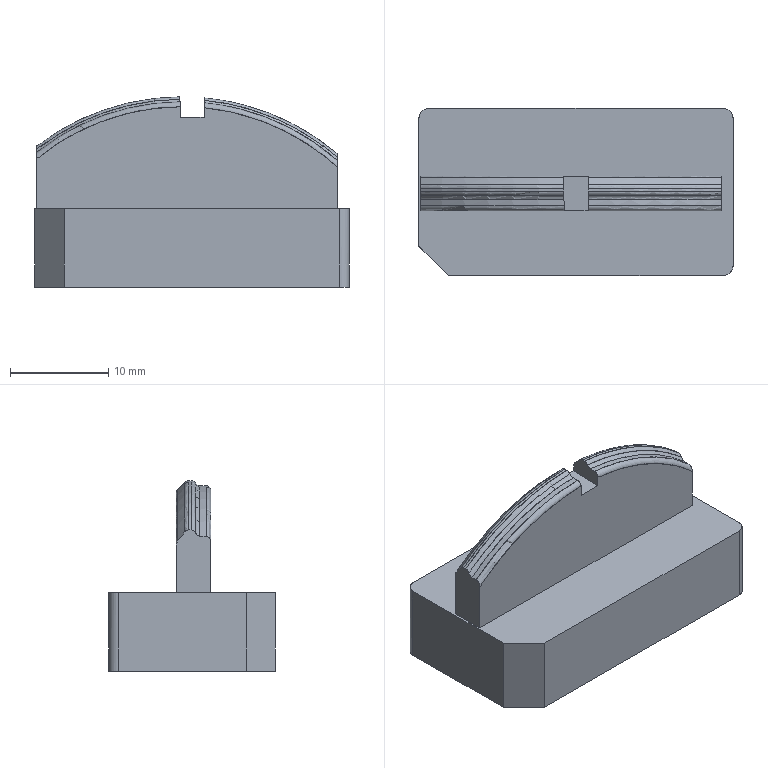NC program | PowerMill | posted with a generic post | part box 32 x 17 x 19.383 mm
Lines 3866 to 4878 of 94163:
N3963 M6
N3964 S18000 M03
N3965 G00 G90 X0.0 Y0.0
N3966 G43 Z9.8028 H2
N3967
N3968 G05 P10000 R4
N3969 X-3.7476 Y3.5833
N3970 Z0.7947
N3971 G01 Z-0.4053 F3600.0
N3972 X-3.7563 Y3.5631 F6000.0
N3973 G03 X-3.6536 Y3.3027 I0.1816 J-0.0788
N3974 G01 X-2.338 Y2.7316
N3975 X-1.4642 Y2.779
N3976 X-0.9761 Y2.7673
N3977 X-0.4881 Y2.6348
N3978 X0.0 Y2.3461
N3979 G03 X0.2177 Y2.3492 I0.1064 J0.1712
N3980 G01 X0.4881 Y2.5054
N3981 X0.9761 Y2.6463
N3982 X1.4642 Y2.6614
N3983 X1.9522 Y2.5817
N3984 X2.4403 Y2.4561
N3985 X2.9283 Y2.272
N3986 X3.0642 Y2.1962
N3987 X3.4164 Y1.9204
N3988 X3.6343 Y1.7082
N3989 X3.9586 Y1.2201
N3990 X4.1158 Y0.7321
N3991 X4.1454 Y0.244
N3992 X4.1238 Y-0.244
N3993 X3.9806 Y-0.7321
N3994 X3.6681 Y-1.2201
N3995 X3.4164 Y-1.4774
N3996 X3.1409 Y-1.7082
N3997 X2.9283 Y-1.8324
N3998 X2.4403 Y-2.0184
N3999 X1.9522 Y-2.1453
N4000 X1.6527 Y-2.1962
N4001 X1.4642 Y-2.2234
N4002 X0.9761 Y-2.2126
N4003 X0.4881 Y-2.076
N4004 X0.1844 Y-1.9036
N4005 X0.0824 Y-1.8775
N4006 X-0.0187 Y-1.9069
N4007 X-0.4881 Y-2.1938
N4008 X-0.9761 Y-2.3211
N4009 X-1.4642 Y-2.3318
N4010 X-2.4403 Y-2.3036
N4011 X-3.9044 Y-2.1592
N4012 X-4.3925 Y-2.0308
N4013 X-4.8805 Y-1.8556
N4014 X-5.134 Y-1.7082
N4015 X-5.6952 Y-1.2201
N4016 X-5.9992 Y-0.7321
N4017 X-6.1407 Y-0.244
N4018 X-6.1636 Y0.244
N4019 X-6.1312 Y0.7321
N4020 X-5.976 Y1.2201
N4021 X-5.6491 Y1.7082
N4022 X-5.3686 Y1.9608
N4023 X-5.0595 Y2.1962
N4024 X-4.8805 Y2.2928
N4025 X-4.3925 Y2.4695
N4026 X-3.9044 Y2.5972
N4027 X-3.2118 Y2.6843
N4028 X-2.338 Y2.7316
N4029 X-3.7478 Y3.8043 Z-0.6036
N4030 X-3.7567 Y3.7842
N4031 G03 X-3.6566 Y3.5227 I0.1808 J-0.0806
N4032 G01 X-2.3471 Y2.9385
N4033 X-1.4642 Y2.9774
N4034 X-0.9761 Y2.965
N4035 X-0.4881 Y2.8316
N4036 X-0.2016 Y2.6843
N4037 X-0.026 Y2.5528
N4038 G03 X0.1946 Y2.5402 I0.1198 J0.1601
N4039 G01 X0.4881 Y2.7114
N4040 X0.9761 Y2.8532
N4041 X1.4642 Y2.8693
N4042 X2.9283 Y2.6859
N4043 X3.4164 Y2.5799
N4044 X3.9044 Y2.4176
N4045 X4.3925 Y2.1844
N4046 X4.8805 Y1.7486
N4047 X5.241 Y1.2201
N4048 X5.3967 Y0.7321
N4049 X5.4278 Y0.244
N4050 X5.4058 Y-0.244
N4051 X5.2581 Y-0.7321
N4052 X4.9589 Y-1.2201
N4053 X4.4471 Y-1.7082
N4054 X3.9044 Y-1.9782
N4055 X3.4164 Y-2.1392
N4056 X3.16 Y-2.1962
N4057 X2.9283 Y-2.2438
N4058 X1.4642 Y-2.3989
N4059 X0.9761 Y-2.3887
N4060 X0.4881 Y-2.2532
N4061 X0.201 Y-2.0907
N4062 X0.0946 Y-2.065
N4063 X-0.0096 Y-2.0985
N4064 X-0.4881 Y-2.3712
N4065 X-0.9761 Y-2.4979
N4066 X-1.4642 Y-2.5012
N4067 X-2.9283 Y-2.4374
N4068 X-4.8805 Y-2.2565
N4069 X-5.1745 Y-2.1962
N4070 X-5.8566 Y-1.9976
N4071 X-6.442 Y-1.7082
N4072 X-6.8327 Y-1.3532
N4073 X-7.2418 Y-0.7321
N4074 X-7.3839 Y-0.244
N4075 X-7.4067 Y0.244
N4076 X-7.3776 Y0.7321
N4077 X-7.2204 Y1.2201
N4078 X-6.9008 Y1.7082
N4079 X-6.3684 Y2.1962
N4080 X-5.8566 Y2.4347
N4081 X-5.3686 Y2.5917
N4082 X-4.9434 Y2.6843
N4083 X-2.9283 Y2.9129
N4084 X-2.3471 Y2.9385
N4085 G00 Z3.3981
N4086 G01 X0.9211 Y-3.7408 F10000.0
N4087 G00 Z0.3981
N4088 G01 Z-0.8019 F3600.0
N4089 X0.9265 Y-3.7195 F6000.0
N4090 G03 X0.7832 Y-3.4789 I-0.1919 J0.0487
N4091 G01 X0.4881 Y-3.404
N4092 X0.2671 Y-3.2865
N4093 G03 X0.0461 Y-3.3086 I-0.0939 J-0.1765
N4094 G01 X0.0 Y-3.3465
N4095 X-0.4881 Y-3.6181
N4096 X-0.6096 Y-3.6604
N4097 X-0.9761 Y-3.7392
N4098 X-1.4642 Y-3.7429
N4099 X-2.4403 Y-3.6987
N4100 X-3.4164 Y-3.5562
N4101 X-3.9044 Y-3.4048
N4102 X-4.2369 Y-3.2391
N4103 X-4.4587 Y-3.7227
N4104 X-4.3614 Y-3.6007
N4105 G03 X-4.4127 Y-3.1454 I-0.2533 J0.2021
N4106 G01 X-4.8805 Y-2.7721
N4107 X-4.9173 Y-2.7232
N4108 X-4.9604 Y-2.6796
N4109 X-5.1023 Y-2.4674
N4110 X-5.1612 Y-2.4098
N4111 X-5.2383 Y-2.3809
N4112 X-6.3447 Y-2.2115
N4113 X-6.8327 Y-2.0687
N4114 X-7.3208 Y-1.836
N4115 X-7.5374 Y-1.7082
N4116 X-7.8088 Y-1.4798
N4117 X-8.0321 Y-1.2201
N4118 X-8.2969 Y-0.7807
N4119 X-8.4632 Y-0.244
N4120 X-8.4838 Y0.244
N4121 X-8.4563 Y0.7321
N4122 X-8.2975 Y1.2201
N4123 X-7.9964 Y1.7082
N4124 X-7.8088 Y1.9185
N4125 X-7.4608 Y2.1962
N4126 X-6.8327 Y2.5063
N4127 X-6.3447 Y2.6533
N4128 X-4.8805 Y2.9144
N4129 X-2.9283 Y3.1355
N4130 X-1.4642 Y3.2002
N4131 X-0.9761 Y3.1871
N4132 X-0.4881 Y3.0526
N4133 X-0.0037 Y2.7633
N4134 X0.0979 Y2.735
N4135 X0.1999 Y2.7624
N4136 X0.4881 Y2.931
N4137 X0.9761 Y3.0739
N4138 X1.4642 Y3.0909
N4139 X2.9283 Y2.9063
N4140 X4.1964 Y2.6843
N4141 X4.8805 Y2.4874
N4142 X5.3686 Y2.2533
N4143 X5.8566 Y1.8745
N4144 X6.0012 Y1.7082
N4145 X6.3138 Y1.2201
N4146 X6.4711 Y0.7321
N4147 X6.5027 Y0.244
N4148 X6.4766 Y-0.244
N4149 X6.3447 Y-0.7097
N4150 X6.0361 Y-1.2201
N4151 X5.8566 Y-1.4383
N4152 X5.5407 Y-1.7082
N4153 X4.8805 Y-2.0491
N4154 X4.3925 Y-2.1953
N4155 X3.9044 Y-2.2952
N4156 X3.2179 Y-2.3924
N4157 X3.1399 Y-2.4209
N4158 X3.0801 Y-2.4786
N4159 X2.9454 Y-2.6783
N4160 X2.673 Y-2.9433
N4161 X4.0519 Y-4.1006 Z-1.0002
N4162 X4.0568 Y-4.0792
N4163 G03 X3.9087 Y-3.8416 I-0.1928 J0.0448
N4164 G01 X2.8287 Y-3.5911
N4165 X2.5403 Y-3.6604
N4166 X1.4642 Y-3.8057
N4167 X0.9761 Y-3.8028
N4168 X0.4582 Y-3.6604
N4169 X0.1659 Y-3.4944
N4170 X0.0607 Y-3.4684
N4171 X-0.0425 Y-3.501
N4172 X-0.2857 Y-3.6604
N4173 X-0.4881 Y-3.7513
N4174 X-0.9761 Y-3.8705
N4175 X-2.4403 Y-3.8583
N4176 X-3.4164 Y-3.8055
N4177 X-4.5237 Y-3.6604
N4178 X-5.3686 Y-3.4189
N4179 X-5.7942 Y-3.1723
N4180 X-6.2938 Y-2.6843
N4181 X-6.4777 Y-2.3999
N4182 X-6.5331 Y-2.3432
N4183 X-6.6062 Y-2.3124
N4184 X-7.1834 Y-2.1962
N4185 X-7.8088 Y-1.9767
N4186 X-8.2543 Y-1.7082
N4187 X-8.7521 Y-1.2201
N4188 X-9.0335 Y-0.7321
N4189 X-9.1759 Y-0.244
N4190 X-9.1994 Y0.244
N4191 X-9.1698 Y0.7321
N4192 X-9.0126 Y1.2201
N4193 X-8.7148 Y1.7082
N4194 X-8.2969 Y2.1169
N4195 X-7.8088 Y2.4151
N4196 X-7.3208 Y2.596
N4197 X-6.3447 Y2.8264
N4198 X-4.8805 Y3.0857
N4199 X-2.9283 Y3.3093
N4200 X-1.4642 Y3.3742
N4201 X-0.9761 Y3.3605
N4202 X-0.4881 Y3.2252
N4203 X-0.3728 Y3.1723
N4204 X-0.0239 Y2.9344
N4205 G03 X0.1902 Y2.9273 I0.1127 J0.1653
N4206 G01 X0.4881 Y3.1025
N4207 X0.9761 Y3.2462
N4208 X1.4642 Y3.264
N4209 X2.9283 Y3.0789
N4210 X5.0066 Y2.6843
N4211 X5.3686 Y2.5799
N4212 X5.8566 Y2.3869
N4213 X6.3447 Y2.0755
N4214 X6.709 Y1.7082
N4215 X6.9935 Y1.2201
N4216 X7.1505 Y0.7321
N4217 X7.1803 Y0.244
N4218 X7.1592 Y-0.244
N4219 X7.0157 Y-0.7321
N4220 X6.7468 Y-1.2201
N4221 X6.3447 Y-1.639
N4222 X5.8566 Y-1.9491
N4223 X5.192 Y-2.1962
N4224 X4.6142 Y-2.3093
N4225 X4.5353 Y-2.3437
N4226 X4.4777 Y-2.4077
N4227 X4.298 Y-2.6843
N4228 X3.7785 Y-3.1723
N4229 X3.4164 Y-3.3918
N4230 X2.9283 Y-3.5672
N4231 X2.8287 Y-3.5911
N4232 X4.0743 Y-4.5766 Z-1.1985
N4233 X4.0829 Y-4.5564
N4234 G03 X3.9773 Y-4.297 I-0.1825 J0.0769
N4235 G01 X2.8435 Y-3.8193
N4236 X1.4642 Y-3.9089
N4237 X0.9761 Y-3.8976
N4238 X0.4881 Y-3.7699
N4239 X0.2603 Y-3.6604
N4240 X0.1365 Y-3.5794
N4241 G03 X-0.0964 Y-3.5886 I-0.1099 J-0.1689
N4242 G01 X-0.2035 Y-3.6604
N4243 X-0.4881 Y-3.7962
N4244 X-0.9761 Y-3.9159
N4245 X-3.4164 Y-3.908
N4246 X-4.8805 Y-3.8231
N4247 X-5.7992 Y-3.6604
N4248 X-6.3447 Y-3.4772
N4249 X-6.9173 Y-3.1723
N4250 X-7.3892 Y-2.6843
N4251 X-7.6086 Y-2.3339
N4252 X-7.6573 Y-2.2806
N4253 X-7.7217 Y-2.2481
N4254 X-8.2969 Y-2.0791
N4255 X-8.7849 Y-1.8369
N4256 X-8.9839 Y-1.7082
N4257 X-9.273 Y-1.4652
N4258 X-9.4825 Y-1.2201
N4259 X-9.7513 Y-0.7321
N4260 X-9.8924 Y-0.244
N4261 X-9.9122 Y0.244
N4262 X-9.8854 Y0.7321
N4263 X-9.7611 Y1.1445
N4264 X-9.4483 Y1.7082
N4265 X-9.273 Y1.9082
N4266 X-8.913 Y2.1962
N4267 X-8.2969 Y2.5187
N4268 X-7.8088 Y2.6786
N4269 X-6.3447 Y3.0215
N4270 X-4.8805 Y3.281
N4271 X-3.4164 Y3.4578
N4272 X-2.4403 Y3.5171
N4273 X-1.4642 Y3.5362
N4274 X-0.9761 Y3.5182
N4275 X-0.4881 Y3.3821
N4276 X-0.1109 Y3.1723
N4277 X-0.0565 Y3.1284
N4278 X0.0039 Y3.0931
N4279 X0.0929 Y3.0806
N4280 X0.1784 Y3.1083
N4281 X0.4881 Y3.2939
N4282 X0.9761 Y3.4385
N4283 X1.4642 Y3.4558
N4284 X2.9283 Y3.2758
N4285 X4.3925 Y3.0063
N4286 X5.8566 Y2.6621
N4287 X6.3447 Y2.5029
N4288 X6.8327 Y2.2505
N4289 X7.3208 Y1.858
N4290 X7.4485 Y1.7082
N4291 X7.7274 Y1.2201
N4292 X7.8829 Y0.7321
N4293 X7.9147 Y0.244
N4294 X7.893 Y-0.244
N4295 X7.8088 Y-0.5812
N4296 X7.4868 Y-1.2201
N4297 X7.3208 Y-1.4233
N4298 X6.9912 Y-1.7082
N4299 X6.3447 Y-2.0633
N4300 X5.9484 Y-2.1962
N4301 X5.7104 Y-2.2531
N4302 X5.6409 Y-2.2847
N4303 X5.5883 Y-2.3401
N4304 X5.3686 Y-2.6844
N4305 X4.9115 Y-3.1723
N4306 X4.3925 Y-3.4629
N4307 X3.8012 Y-3.6604
N4308 X2.9283 Y-3.8138
N4309 X2.8435 Y-3.8193
N4310 X4.2618 Y-4.7703 Z-1.3968
N4311 X4.2707 Y-4.7502
N4312 G03 X4.1701 Y-4.4888 I-0.181 J0.0804
N4313 G01 X2.8473 Y-3.9016
N4314 X2.4403 Y-3.9202
N4315 X0.9761 Y-3.9125
N4316 X0.4881 Y-3.7842
N4317 X0.2344 Y-3.6604
N4318 X0.1276 Y-3.5888
N4319 G03 X-0.0947 Y-3.5886 I-0.1113 J-0.1662
N4320 G01 X-0.2024 Y-3.6604
N4321 X-0.4881 Y-3.7968
N4322 X-0.9761 Y-3.9164
N4323 X-3.9044 Y-3.9296
N4324 X-4.8805 Y-3.9084
N4325 X-5.8566 Y-3.8352
N4326 X-6.7635 Y-3.6604
N4327 X-7.3208 Y-3.4436
N4328 X-7.7947 Y-3.1723
N4329 X-8.2533 Y-2.6843
N4330 X-8.4847 Y-2.3001
N4331 X-8.5245 Y-2.2523
N4332 X-8.5781 Y-2.2208
N4333 X-8.6012 Y-2.2109
N4334 X-8.6527 Y-2.1962
N4335 X-9.273 Y-1.9379
N4336 X-9.7611 Y-1.5971
N4337 X-10.108 Y-1.2201
N4338 X-10.3725 Y-0.7321
N4339 X-10.5159 Y-0.244
N4340 X-10.537 Y0.244
N4341 X-10.5061 Y0.7321
N4342 X-10.3494 Y1.2201
N4343 X-10.2491 Y1.4287
N4344 X-10.0737 Y1.7082
N4345 X-9.7611 Y2.0328
N4346 X-9.273 Y2.3756
N4347 X-8.7849 Y2.5868
N4348 X-8.2969 Y2.7377
N4349 X-6.3447 Y3.2166
N4350 X-5.3686 Y3.3922
N4351 X-4.3925 Y3.5187
N4352 X-3.4164 Y3.5695
N4353 X-1.4642 Y3.5905
N4354 X-0.9761 Y3.5691
N4355 X-0.4881 Y3.4328
N4356 X-0.0774 Y3.1815
N4357 X0.0273 Y3.152
N4358 X0.1319 Y3.1818
N4359 X0.4881 Y3.4013
N4360 X0.9761 Y3.5464
N4361 X1.4642 Y3.5679
N4362 X2.4403 Y3.5173
N4363 X3.4164 Y3.3891
N4364 X4.5405 Y3.1723
N4365 X6.3447 Y2.7263
N4366 X6.8327 Y2.5705
N4367 X7.3208 Y2.3465
N4368 X7.8088 Y1.9922
N4369 X8.0731 Y1.7082
N4370 X8.3563 Y1.2201
N4371 X8.5112 Y0.7321
N4372 X8.5444 Y0.244
N4373 X8.5208 Y-0.244
N4374 X8.3776 Y-0.7321
N4375 X8.1095 Y-1.2201
N4376 X7.8088 Y-1.5521
N4377 X7.3208 Y-1.9106
N4378 X6.8327 Y-2.1283
N4379 X6.6164 Y-2.2014
N4380 X6.5529 Y-2.2368
N4381 X6.5063 Y-2.2925
N4382 X6.3447 Y-2.5786
N4383 X5.8566 Y-3.1312
N4384 X5.3686 Y-3.4257
N4385 X4.7624 Y-3.6604
N4386 X3.9044 Y-3.8298
N4387 X3.4164 Y-3.8755
N4388 X2.8473 Y-3.9016
N4389 X4.2549 Y-4.8818 Z-1.5951
N4390 X4.2649 Y-4.8622
N4391 G03 X4.1777 Y-4.5961 I-0.1767 J0.0895
N4392 G01 X2.8472 Y-3.9222
N4393 X2.4423 Y-3.9201
N4394 X2.4403 Y-3.9202
N4395 X1.5735 Y-3.9156
N4396 X0.9761 Y-3.9125
N4397 X0.4881 Y-3.7842
N4398 X0.2344 Y-3.6604
N4399 X0.1276 Y-3.5888
N4400 G03 X-0.0947 Y-3.5886 I-0.1113 J-0.1662
N4401 G01 X-0.2023 Y-3.6604
N4402 X-0.4881 Y-3.7969
N4403 X-0.9761 Y-3.9165
N4404 X-1.4642 Y-3.9296
N4405 X-3.6604 Y-3.9248
N4406 X-5.8566 Y-3.9121
N4407 X-6.8327 Y-3.8243
N4408 X-7.3208 Y-3.7294
N4409 X-7.8088 Y-3.5861
N4410 X-8.2969 Y-3.3434
N4411 X-8.5615 Y-3.1723
N4412 X-8.7849 Y-2.9711
N4413 X-9.0165 Y-2.6843
N4414 X-9.2792 Y-2.2399
N4415 X-9.3211 Y-2.19
N4416 X-9.3768 Y-2.1561
N4417 X-9.7611 Y-2.0017
N4418 X-10.2491 Y-1.6931
N4419 X-10.7134 Y-1.2201
N4420 X-10.9673 Y-0.7321
N4421 X-11.1069 Y-0.244
N4422 X-11.127 Y0.244
N4423 X-11.0949 Y0.7321
N4424 X-10.946 Y1.2201
N4425 X-10.6744 Y1.7082
N4426 X-10.2491 Y2.1292
N4427 X-9.7611 Y2.4407
N4428 X-9.273 Y2.6317
N4429 X-8.2969 Y2.9268
N4430 X-6.3447 Y3.4101
N4431 X-5.3686 Y3.5364
N4432 X-4.3925 Y3.5845
N4433 X-1.4642 Y3.5944
N4434 X-0.9761 Y3.5716
N4435 X-0.4881 Y3.436
N4436 X-0.0887 Y3.1932
N4437 X0.0159 Y3.1641
N4438 X0.1202 Y3.1939
N4439 X0.4881 Y3.421
N4440 X0.9761 Y3.5596
N4441 X1.4642 Y3.5944
N4442 X1.9522 Y3.5919
N4443 X3.4164 Y3.5345
N4444 X4.3925 Y3.396
N4445 X5.8566 Y3.0431
N4446 X7.3208 Y2.62
N4447 X7.8088 Y2.4184
N4448 X8.1649 Y2.1962
N4449 X8.6716 Y1.7082
N4450 X8.7849 Y1.5404
N4451 X8.9458 Y1.2201
N4452 X9.0987 Y0.7321
N4453 X9.129 Y0.244
N4454 X9.1075 Y-0.244
N4455 X8.9656 Y-0.7321
N4456 X8.7083 Y-1.2201
N4457 X8.2969 Y-1.6507
N4458 X7.8088 Y-1.9803
N4459 X7.3504 Y-2.1652
N4460 X7.2925 Y-2.201
N4461 X7.25 Y-2.2542
N4462 X7.0133 Y-2.6843
N4463 X6.8327 Y-2.9175
N4464 X6.5586 Y-3.1723
N4465 X6.3447 Y-3.313
N4466 X5.8566 Y-3.5641
N4467 X5.5713 Y-3.6604
N4468 X4.8805 Y-3.8203
N4469 X4.3925 Y-3.8741
N4470 X3.4164 Y-3.9251
N4471 X2.8472 Y-3.9222
N4472 X4.2768 Y-4.8954 Z-1.7934
N4473 X4.2868 Y-4.8757
N4474 G03 X4.1998 Y-4.6096 I-0.1766 J0.0895
N4475 G01 X2.8471 Y-3.9234
N4476 X0.9761 Y-3.9125
N4477 X0.4881 Y-3.7843
N4478 X0.2343 Y-3.6604
N4479 X0.1276 Y-3.5888
N4480 G03 X-0.0948 Y-3.5886 I-0.1114 J-0.1662
N4481 G01 X-0.2023 Y-3.6604
N4482 X-0.4881 Y-3.7969
N4483 X-0.9761 Y-3.9165
N4484 X-1.4642 Y-3.9296
N4485 X-5.3686
N4486 X-6.8327 Y-3.9071
N4487 X-7.8088 Y-3.7873
N4488 X-8.2969 Y-3.6577
N4489 X-8.7849 Y-3.4585
N4490 X-9.2589 Y-3.1723
N4491 X-9.7149 Y-2.6843
N4492 X-9.9607 Y-2.2037
N4493 X-10.001 Y-2.1498
N4494 X-10.0568 Y-2.1123
N4495 X-10.2491 Y-2.0258
N4496 X-10.7372 Y-1.7285
N4497 X-11.2434 Y-1.2201
N4498 X-11.4976 Y-0.7321
N4499 X-11.6375 Y-0.244
N4500 X-11.6595 Y0.244
N4501 X-11.6292 Y0.7321
N4502 X-11.4793 Y1.2201
N4503 X-11.2252 Y1.683
N4504 X-10.7372 Y2.1655
N4505 X-10.2491 Y2.4644
N4506 X-9.7611 Y2.6661
N4507 X-8.1071 Y3.1723
N4508 X-7.3208 Y3.3765
N4509 X-6.8327 Y3.475
N4510 X-6.3447 Y3.5354
N4511 X-5.3686 Y3.5887
N4512 X-1.4642 Y3.5944
N4513 X-0.9761 Y3.5742
N4514 X-0.4881 Y3.4391
N4515 X-0.0896 Y3.1944
N4516 G03 X0.1327 Y3.2024 I0.105 J0.172
N4517 G01 X0.4881 Y3.4246
N4518 X0.9761 Y3.5623
N4519 X1.4642 Y3.5944
N4520 X1.4758 Y3.5942
N4521 X1.9522 Y3.5919
N4522 X2.0243 Y3.589
N4523 X3.9044 Y3.5712
N4524 X4.8805 Y3.4645
N4525 X6.1004 Y3.1723
N4526 X7.8088 Y2.6455
N4527 X8.2969 Y2.4419
N4528 X8.6998 Y2.1962
N4529 X9.2068 Y1.7082
N4530 X9.4883 Y1.2201
N4531 X9.6444 Y0.7321
N4532 X9.6778 Y0.244
N4533 X9.6535 Y-0.244
N4534 X9.5108 Y-0.7321
N4535 X9.273 Y-1.1713
N4536 X8.7618 Y-1.7082
N4537 X8.2969 Y-2.0031
N4538 X8.0623 Y-2.109
N4539 X8.0083 Y-2.1449
N4540 X7.9686 Y-2.1963
N4541 X7.7051 Y-2.6843
N4542 X7.3208 Y-3.114
N4543 X6.8327 Y-3.438
N4544 X6.292 Y-3.6604
N4545 X5.8566 Y-3.776
N4546 X4.8805 Y-3.9048
N4547 X3.9044 Y-3.9296
N4548 X2.8471 Y-3.9234
N4549 X4.2769 Y-4.8954 Z-1.9917
N4550 X4.2869 Y-4.8757
N4551 G03 X4.1999 Y-4.6096 I-0.1766 J0.0895
N4552 G01 X2.8471 Y-3.9234
N4553 X1.0244 Y-3.9128
N4554 X0.9761 Y-3.9125
N4555 X0.4881 Y-3.7843
N4556 X0.2343 Y-3.6604
N4557 X0.1276 Y-3.5889
N4558 G03 X-0.0948 Y-3.5886 I-0.1114 J-0.1661
N4559 G01 X-0.2023 Y-3.6604
N4560 X-0.4881 Y-3.7969
N4561 X-0.9761 Y-3.9165
N4562 X-1.4642 Y-3.9296
N4563 X-6.8327
N4564 X-7.8088 Y-3.8901
N4565 X-8.2969 Y-3.8226
N4566 X-8.7849 Y-3.7041
N4567 X-9.273 Y-3.5292
N4568 X-9.852 Y-3.1723
N4569 X-10.2491 Y-2.7656
N4570 X-10.5796 Y-2.156
N4571 X-10.6133 Y-2.1106
N4572 X-10.6583 Y-2.0764
N4573 X-11.2252 Y-1.7615
N4574 X-11.7133 Y-1.2846
N4575 X-12.0174 Y-0.7321
N4576 X-12.1572 Y-0.244
N4577 X-12.1798 Y0.244
N4578 X-12.1485 Y0.7321
N4579 X-11.9967 Y1.2201
N4580 X-11.7133 Y1.7213
N4581 X-11.235 Y2.1962
N4582 X-10.7372 Y2.4829
N4583 X-9.7611 Y2.8517
N4584 X-8.2969 Y3.3044
N4585 X-7.8088 Y3.4319
N4586 X-7.3208 Y3.5174
N4587 X-6.8327 Y3.5691
N4588 X-5.8566 Y3.5944
N4589 X-1.4642
N4590 X-0.9761 Y3.5767
N4591 X-0.4881 Y3.4423
N4592 X-0.0906 Y3.1957
N4593 G03 X0.1218 Y3.1966 I0.1054 J0.1699
N4594 G01 X0.4881 Y3.4282
N4595 X0.9761 Y3.565
N4596 X1.4642 Y3.5944
N4597 X4.3925 Y3.5865
N4598 X5.3686 Y3.5133
N4599 X5.8566 Y3.4211
N4600 X6.3447 Y3.2943
N4601 X7.8088 Y2.8338
N4602 X8.7849 Y2.4643
N4603 X9.2341 Y2.1962
N4604 X9.7236 Y1.7082
N4605 X9.9958 Y1.2201
N4606 X10.141 Y0.7321
N4607 X10.1705 Y0.244
N4608 X10.1504 Y-0.244
N4609 X10.0156 Y-0.7321
N4610 X9.7619 Y-1.2201
N4611 X9.2951 Y-1.7082
N4612 X8.7849 Y-2.0239
N4613 X8.7048 Y-2.0578
N4614 X8.6289 Y-2.1003
N4615 X8.5968 Y-2.1309
N4616 X8.5722 Y-2.1678
N4617 X8.3053 Y-2.6843
N4618 X7.8533 Y-3.1723
N4619 X7.3208 Y-3.502
N4620 X6.9187 Y-3.6604
N4621 X6.3447 Y-3.8134
N4622 X5.8566 Y-3.8849
N4623 X4.8805 Y-3.9296
N4624 X4.0459 Y-3.9259
N4625 X4.043 Y-3.926
N4626 X3.9044 Y-3.9295
N4627 X2.8471 Y-3.9234
N4628 X4.2856 Y-4.8948 Z-2.19
N4629 X4.2955 Y-4.8751
N4630 G03 X4.2069 Y-4.6095 I-0.1771 J0.0886
N4631 G01 X2.8471 Y-3.9296
N4632 X1.4642
N4633 X0.9761 Y-3.9126
N4634 X0.4881 Y-3.7843
N4635 X0.2343 Y-3.6604
N4636 X0.1276 Y-3.5889
N4637 G03 X-0.1069 Y-3.5967 I-0.1118 J-0.1678
N4638 G01 X-0.2023 Y-3.6604
N4639 X-0.4881 Y-3.7969
N4640 X-0.9761 Y-3.9165
N4641 X-1.4642 Y-3.9296
N4642 X-6.8327
N4643 X-8.2969 Y-3.9028
N4644 X-8.7849 Y-3.8387
N4645 X-9.273 Y-3.737
N4646 X-9.7611 Y-3.5742
N4647 X-10.2491 Y-3.3018
N4648 X-10.4294 Y-3.1723
N4649 X-10.7372 Y-2.8758
N4650 X-10.8833 Y-2.6843
N4651 X-11.1506 Y-2.1227
N4652 X-11.1833 Y-2.0741
N4653 X-11.2286 Y-2.037
N4654 X-11.7133 Y-1.7472
N4655 X-12.2013 Y-1.2552
N4656 X-12.4848 Y-0.7321
N4657 X-12.623 Y-0.244
N4658 X-12.6482 Y0.244
N4659 X-12.6165 Y0.7321
N4660 X-12.4627 Y1.2201
N4661 X-12.1893 Y1.7082
N4662 X-11.7011 Y2.1962
N4663 X-11.2252 Y2.4844
N4664 X-9.7611 Y3.0374
N4665 X-8.7849 Y3.3487
N4666 X-8.2969 Y3.4687
N4667 X-7.8088 Y3.5435
N4668 X-6.8327 Y3.5944
N4669 X-1.4642
N4670 X-0.9761 Y3.5792
N4671 X-0.4881 Y3.4454
N4672 X-0.0915 Y3.1968
N4673 G03 X0.1226 Y3.1979 I0.1063 J0.1695
N4674 G01 X0.4881 Y3.4319
N4675 X0.9761 Y3.5677
N4676 X1.4642 Y3.5944
N4677 X4.8805
N4678 X5.8566 Y3.5364
N4679 X6.3447 Y3.4588
N4680 X6.8327 Y3.3399
N4681 X7.8105 Y3.009
N4682 X8.7849 Y2.6683
N4683 X9.273 Y2.4547
N4684 X9.7002 Y2.1962
N4685 X10.1899 Y1.7082
N4686 X10.4621 Y1.2201
N4687 X10.6073 Y0.7321
N4688 X10.6367 Y0.244
N4689 X10.6131 Y-0.244
N4690 X10.4795 Y-0.7321
N4691 X10.2491 Y-1.1834
N4692 X9.7611 Y-1.7085
N4693 X9.2306 Y-2.0345
N4694 X9.1872 Y-2.0705
N4695 X9.1556 Y-2.1173
N4696 X8.8793 Y-2.6843
N4697 X8.7849 Y-2.8136
N4698 X8.4237 Y-3.1723
N4699 X7.8088 Y-3.5564
N4700 X7.5194 Y-3.6604
N4701 X6.8327 Y-3.8306
N4702 X6.3447 Y-3.8998
N4703 X5.3686 Y-3.9296
N4704 X2.8471
N4705 X4.2785 Y-4.8912 Z-2.3883
N4706 X4.2884 Y-4.8715
N4707 G03 X4.1998 Y-4.6059 I-0.1771 J0.0886
N4708 G01 X2.8471 Y-3.9295
N4709 X1.4639
N4710 X-8.2969 Y-3.9296
N4711 X-8.7849 Y-3.9088
N4712 X-9.273 Y-3.8559
N4713 X-9.7611 Y-3.7584
N4714 X-10.2491 Y-3.5878
N4715 X-10.7372 Y-3.317
N4716 X-10.9389 Y-3.1723
N4717 X-11.2252 Y-2.9018
N4718 X-11.3924 Y-2.6843
N4719 X-11.6702 Y-2.0935
N4720 X-11.7021 Y-2.0453
N4721 X-11.7464 Y-2.0082
N4722 X-12.2013 Y-1.7284
N4723 X-12.6901 Y-1.2201
N4724 X-12.9444 Y-0.7321
N4725 X-13.0795 Y-0.244
N4726 X-13.0995 Y0.244
N4727 X-13.0699 Y0.7321
N4728 X-12.9259 Y1.2201
N4729 X-12.6894 Y1.6592
N4730 X-12.2013 Y2.1662
N4731 X-11.7133 Y2.4736
N4732 X-11.2202 Y2.6843
N4733 X-9.273 Y3.3836
N4734 X-8.7849 Y3.4977
N4735 X-8.2969 Y3.5609
N4736 X-7.3208 Y3.5944
N4737 X5.3686
N4738 X6.3447 Y3.5568
N4739 X6.8327 Y3.4886
N4740 X7.3208 Y3.3658
N4741 X8.7849 Y2.8504
N4742 X9.7611 Y2.4452
N4743 X10.1662 Y2.1962
N4744 X10.6557 Y1.7082
N4745 X10.9259 Y1.2201
N4746 X11.0709 Y0.7321
N4747 X11.1012 Y0.244
N4748 X11.0759 Y-0.244
N4749 X10.9434 Y-0.7321
N4750 X10.69 Y-1.2201
N4751 X10.2247 Y-1.7082
N4752 X9.7726 Y-1.9928
N4753 X9.7306 Y-2.0278
N4754 X9.701 Y-2.0737
N4755 X9.6912 Y-2.0935
N4756 X9.6538 Y-2.1962
N4757 X9.3916 Y-2.6843
N4758 X9.273 Y-2.844
N4759 X8.9366 Y-3.1723
N4760 X8.2969 Y-3.5669
N4761 X8.0479 Y-3.6604
N4762 X7.8088 Y-3.7445
N4763 X7.3208 Y-3.8482
N4764 X6.8327 Y-3.9062
N4765 X6.3447 Y-3.9295
N4766 X5.3692
N4767 X5.3686
N4768 X2.8471
N4769 X4.2851 Y-4.8945 Z-2.5866
N4770 X4.295 Y-4.8748
N4771 G03 X4.2064 Y-4.6092 I-0.1771 J0.0885
N4772 G01 X2.8471 Y-3.9296
N4773 X-8.7849
N4774 X-9.273 Y-3.9127
N4775 X-9.7611 Y-3.8614
N4776 X-10.2491 Y-3.7642
N4777 X-10.7372 Y-3.5969
N4778 X-11.2252 Y-3.3325
N4779 X-11.4401 Y-3.1723
N4780 X-11.7133 Y-2.9206
N4781 X-11.897 Y-2.6843
N4782 X-12.1389 Y-2.1962
N4783 X-12.186 Y-2.0642
N4784 X-12.217 Y-2.0081
N4785 X-12.264 Y-1.9647
N4786 X-12.6516 Y-1.7082
N4787 X-13.1036 Y-1.2201
N4788 X-13.3592 Y-0.7321
N4789 X-13.4975 Y-0.244
N4790 X-13.518 Y0.244
N4791 X-13.4884 Y0.7321
N4792 X-13.3388 Y1.2201
N4793 X-13.1774 Y1.5458
N4794 X-13.0676 Y1.7082
N4795 X-12.6894 Y2.1136
N4796 X-12.2013 Y2.443
N4797 X-11.2252 Y2.8655
N4798 X-9.7611 Y3.3971
N4799 X-9.273 Y3.5085
N4800 X-8.7849 Y3.572
N4801 X-8.2969 Y3.5925
N4802 X-7.3695 Y3.5926
N4803 X-7.3662 Y3.5928
N4804 X-7.3208 Y3.5943
N4805 X4.9828
N4806 X5.3686 Y3.5944
N4807 X6.8327 Y3.5677
N4808 X7.3208 Y3.5027
N4809 X7.8088 Y3.3859
N4810 X9.7611 Y2.6483
N4811 X10.2491 Y2.4165
N4812 X10.5905 Y2.1962
N4813 X10.7372 Y2.0684
N4814 X11.0669 Y1.7082
N4815 X11.2252 Y1.4625
N4816 X11.338 Y1.2201
N4817 X11.486 Y0.7321
N4818 X11.5159 Y0.244
N4819 X11.4939 Y-0.244
N4820 X11.3586 Y-0.7321
N4821 X11.2252 Y-1.0229
N4822 X11.1038 Y-1.2201
N4823 X10.7372 Y-1.6317
N4824 X10.2525 Y-1.9692
N4825 X10.2078 Y-2.012
N4826 X10.1783 Y-2.0664
N4827 X10.1321 Y-2.1962
N4828 X9.8946 Y-2.6843
N4829 X9.7611 Y-2.862
N4830 X9.4404 Y-3.1723
N4831 X9.273 Y-3.3004
N4832 X8.7849 Y-3.5789
N4833 X8.5613 Y-3.6604
N4834 X8.2969 Y-3.7514
N4835 X7.8088 Y-3.8523
N4836 X7.3208 Y-3.9097
N4837 X6.8327 Y-3.9296
N4838 X2.8471
N4839 X4.2859 Y-4.8949 Z-2.7849
N4840 X4.2957 Y-4.8752
N4841 G03 X4.2072 Y-4.6096 I-0.1771 J0.0885
N4842 G01 X2.8471 Y-3.9296
N4843 X-9.273
N4844 X-9.7611 Y-3.9139
N4845 X-10.2491 Y-3.8654
N4846 X-10.7372 Y-3.7666
N4847 X-11.2252 Y-3.5845
N4848 X-11.7133 Y-3.3105
N4849 X-12.2013 Y-2.8704
N4850 X-12.3414 Y-2.6843
N4851 X-12.5854 Y-2.1962
N4852 X-12.6397 Y-2.0397
N4853 X-12.6473 Y-2.0257
N4854 X-12.6753 Y-1.9767
N4855 X-12.7173 Y-1.9391
N4856 X-13.062 Y-1.7082
N4857 X-13.514 Y-1.2201
N4858 X-13.6655 Y-0.966
N4859 X-13.7688 Y-0.7321
N4860 X-13.9068 Y-0.244
N4861 X-13.9306 Y0.244
N4862 X-13.899 Y0.7321
N4863 X-13.7516 Y1.2201
N4864 X-13.6655 Y1.4101
N4865 X-13.4797 Y1.7082
N4866 X-13.1774 Y2.0422
N4867 X-13.0031 Y2.1962
N4868 X-12.6894 Y2.4001
N4869 X-11.2252 Y3.0497
N4870 X-10.2491 Y3.4049
N4871 X-9.7611 Y3.5157
N4872 X-9.273 Y3.5746
N4873 X-8.7849 Y3.5944
N4874 X-2.9893 Y3.5943
N4875 X4.9828
N4876 X5.3686
N4877 X5.3799 Y3.5941
N4878 X6.8327
N4879 X7.3208 Y3.5728
N4880 X7.8088 Y3.5075
N4881 X8.2969 Y3.3916
N4882 X8.7849 Y3.2136
N4883 X10.1039 Y2.6843
N4884 X10.7372 Y2.373
N4885 X11.0009 Y2.1962
N4886 X11.2252 Y1.991
N4887 X11.4772 Y1.7082
N4888 X11.7133 Y1.3037
N4889 X11.8932 Y0.7321
N4890 X11.9229 Y0.244
N4891 X11.8998 Y-0.244
N4892 X11.7674 Y-0.7321
N4893 X11.5117 Y-1.2201
N4894 X11.0614 Y-1.7082
N4895 X10.7087 Y-1.9435
N4896 X10.6618 Y-1.9872
N4897 X10.6311 Y-2.0435
N4898 X10.5773 Y-2.1962
N4899 X10.3405 Y-2.6843
N4900 X10.2491 Y-2.8094
N4901 X9.7611 Y-3.2719
N4902 X9.273 Y-3.5642
N4903 X9.0312 Y-3.6642
N4904 X8.7849 Y-3.7528
N4905 X8.2969 Y-3.8569
N4906 X7.8088 Y-3.9115
N4907 X7.3208 Y-3.9296
N4908 X2.8471
N4909 X4.2783 Y-4.8911 Z-2.9832
N4910 X4.2881 Y-4.8714
N4911 G03 X4.1996 Y-4.6058 I-0.1771 J0.0885
N4912 G01 X2.8471 Y-3.9296
N4913 X-9.7611
N4914 X-10.2491 Y-3.9146
N4915 X-10.7372 Y-3.8627
N4916 X-11.2252 Y-3.7547
N4917 X-11.7133 Y-3.5668
N4918 X-12.2013 Y-3.2767
N4919 X-12.6894 Y-2.8186
N4920 X-12.7859 Y-2.6843
N4921 X-13.025 Y-2.1962
N4922 X-13.0853 Y-2.0187
N4923 X-13.1199 Y-1.9565
N4924 X-13.1736 Y-1.9098
N4925 X-13.464 Y-1.7082
N4926 X-13.6655 Y-1.5098
N4927 X-13.9059 Y-1.2201
N4928 X-14.159 Y-0.7321
N4929 X-14.2874 Y-0.244
N4930 X-14.3069 Y0.244
N4931 X-14.2773 Y0.7321
N4932 X-14.1395 Y1.2201
N4933 X-13.8677 Y1.7082
N4934 X-13.6655 Y1.9442
N4935 X-13.4005 Y2.1962
N4936 X-13.1774 Y2.3492
N4937 X-12.6894 Y2.6033
N4938 X-11.2252 Y3.2315
N4939 X-10.7372 Y3.4009
N4940 X-10.2491 Y3.5148
N4941 X-9.7611 Y3.5765
N4942 X-9.273 Y3.5944
N4943 X7.3208
N4944 X7.8088 Y3.5734
N4945 X8.2969 Y3.5083
N4946 X8.7849 Y3.3883
N4947 X9.273 Y3.2131
N4948 X10.7372 Y2.5838
N4949 X11.2252 Y2.3191
N4950 X11.4022 Y2.1962
N4951 X11.8685 Y1.7082
N4952 X12.1405 Y1.2201
N4953 X12.2818 Y0.7321
N4954 X12.3117 Y0.244
N4955 X12.292 Y-0.244
N4956 X12.1602 Y-0.7321
N4957 X11.9069 Y-1.2201
N4958 X11.4655 Y-1.7082
N4959 X11.1645 Y-1.9153
N4960 X11.119 Y-1.9585
N4961 X11.0892 Y-2.0136
N4962 X10.7864 Y-2.6843
N4963 X10.3308 Y-3.1723
N4964 X9.7611 Y-3.547
N4965 X9.5186 Y-3.6477
N4966 X9.273 Y-3.7405
N4967 X8.7849 Y-3.8523
N4968 X8.2969 Y-3.9112
N4969 X7.8088 Y-3.9296
N4970 X2.8471
N4971 X4.2859 Y-4.8949 Z-3.1815
N4972 X4.2957 Y-4.8752
N4973 G03 X4.2072 Y-4.6096 I-0.177 J0.0885
N4974 G01 X2.8471 Y-3.9296
N4975 X-10.2491